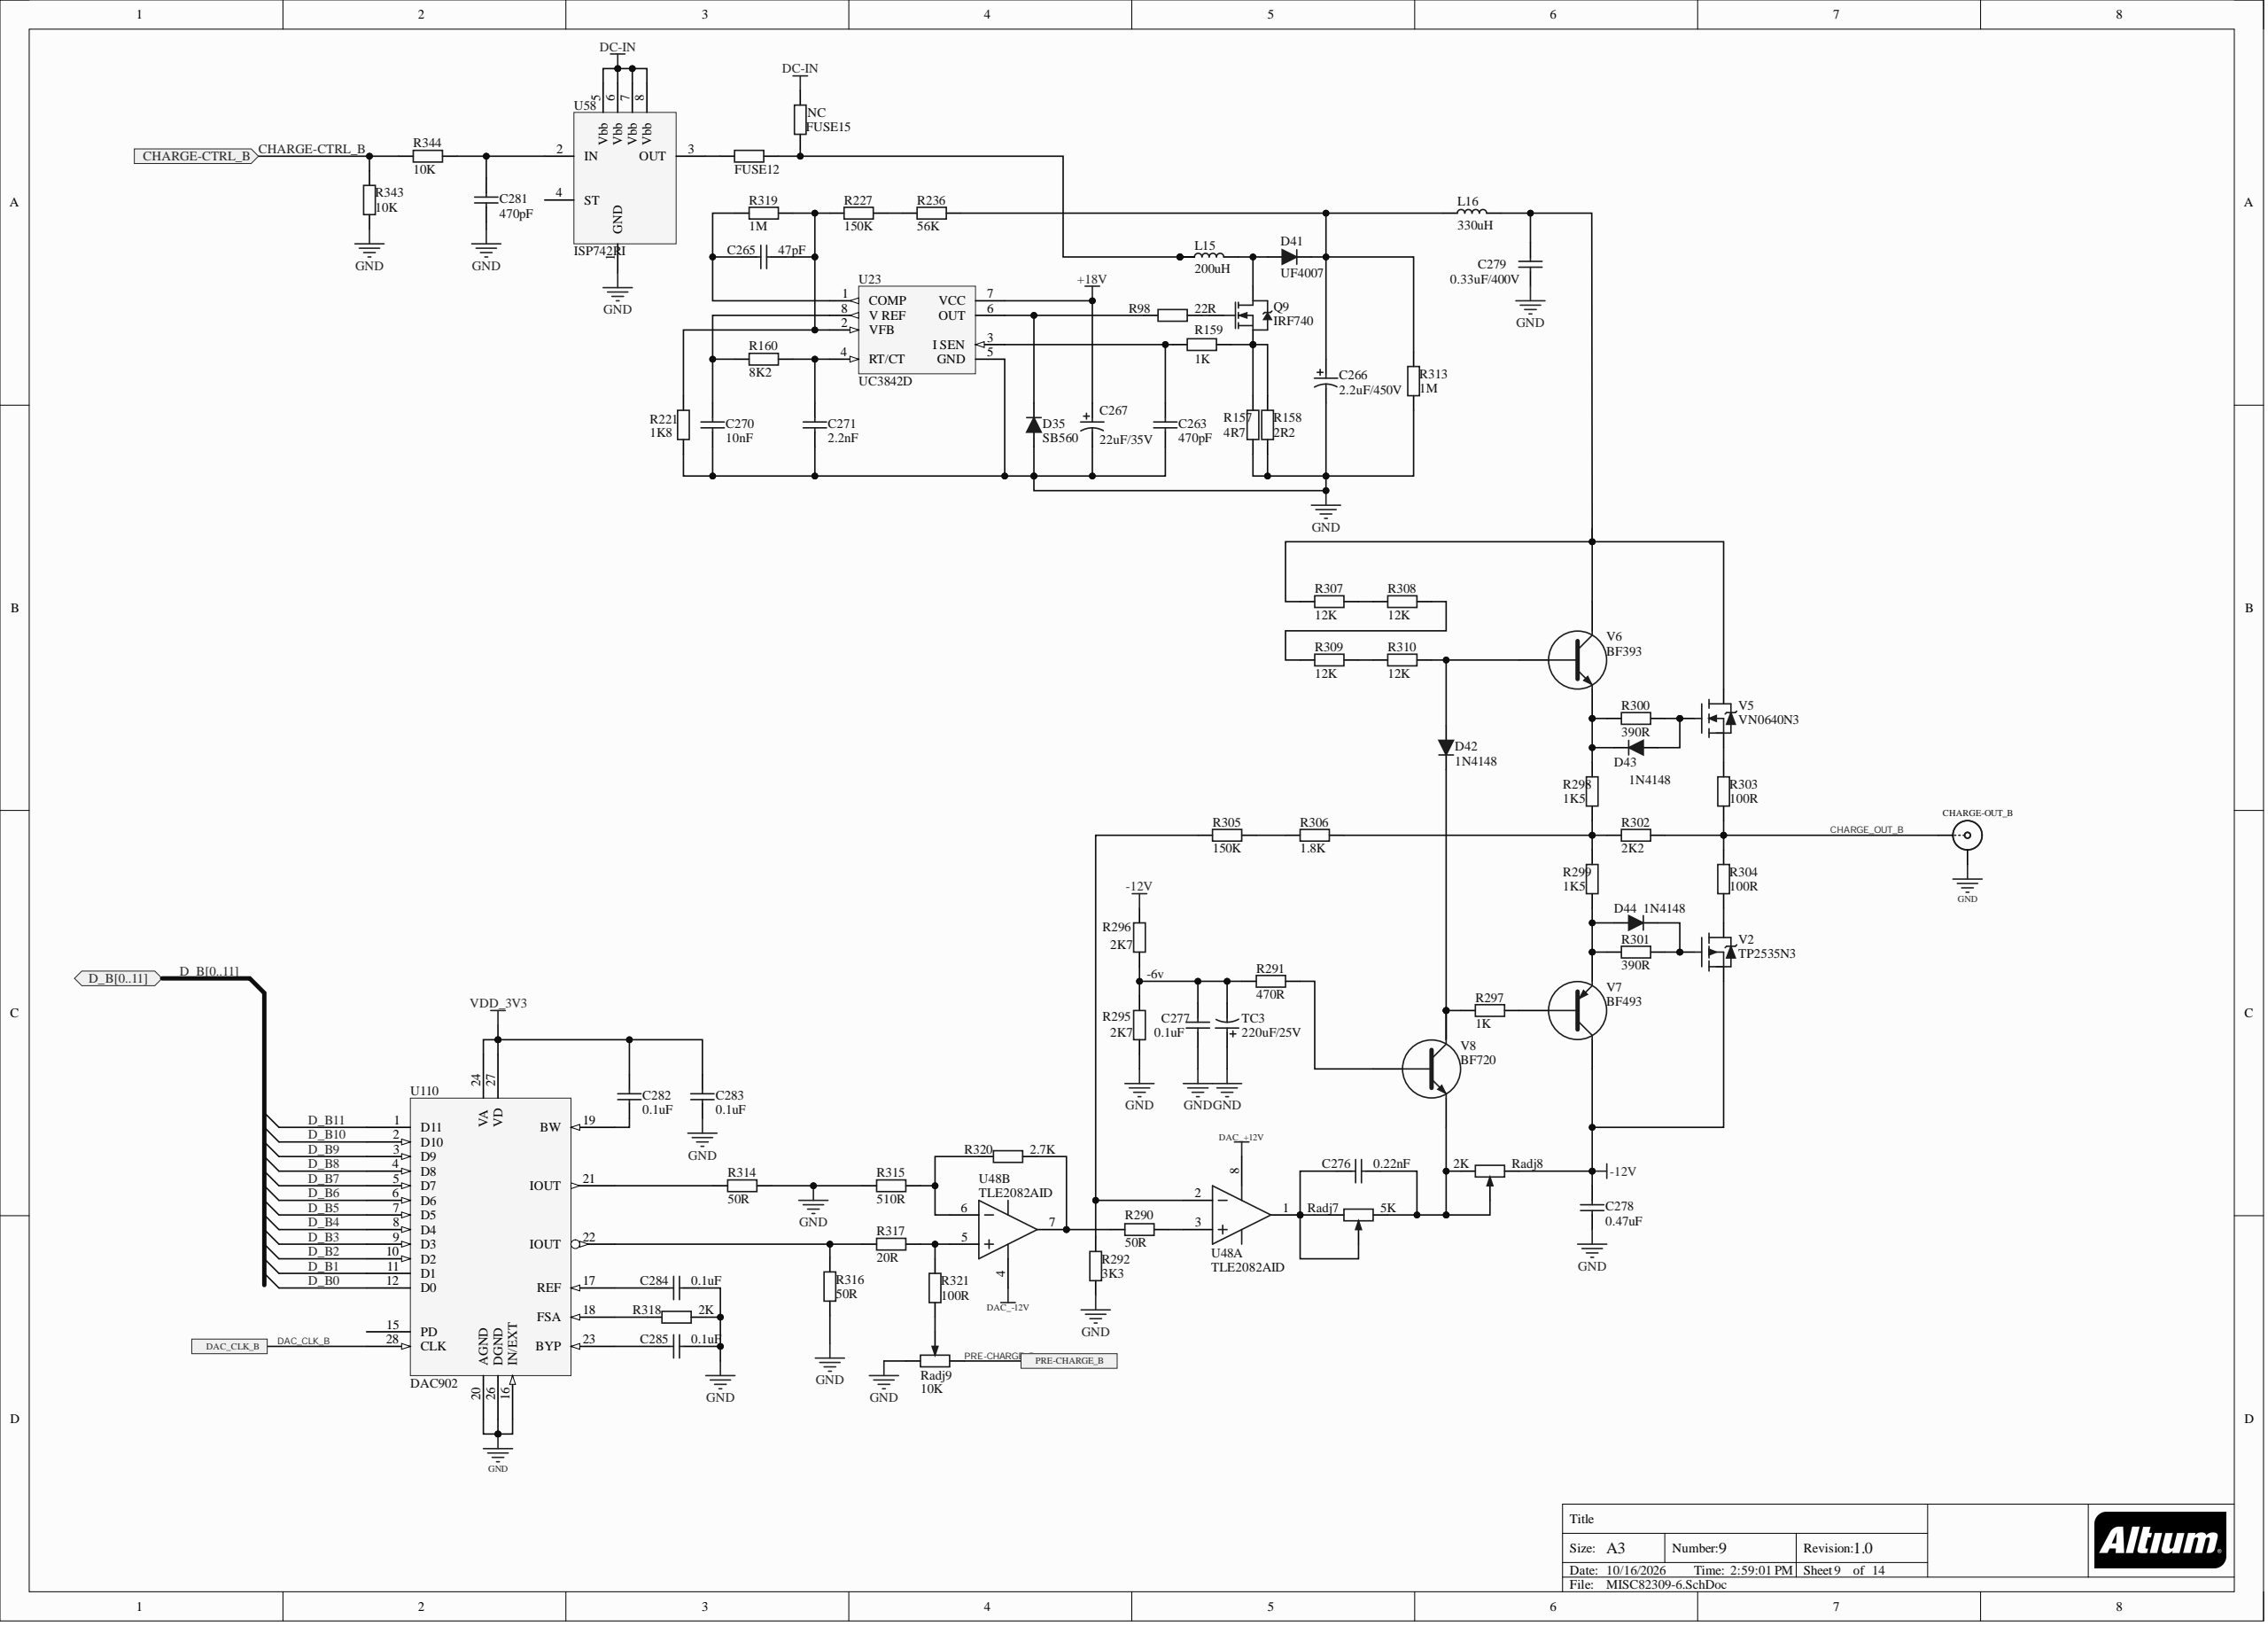Circuit board | Altium Designer | 747 parts | 576 nets | one sheet of the schematic
Parts on this sheet (reference | value | footprint):
C263 | 470pF | C1206
C265 | 47pF | C1206
C266 | 2.2uF/450V | CAP-EL-10X13_5-5
C267 | 22uF/35V | E6.3X5.4
C270 | 10nF | C1206
C271 | 2.2nF | C1206
C276 | 0.22nF | CAP_0805
C277 | 0.1uF | CAP_0805
C278 | 0.47uF | C1206
C279 | 0.33uF/400V | CBB-400V-10mm
C281 | 470pF | C0603
C282 | 0.1uF | CAP_0805
C283 | 0.1uF | CAP_0805
C284 | 0.1uF | CAP_0805
C285 | 0.1uF | CAP_0805
CHARGE-OUT_B | SMB | SMB_V-RJ45
D35 | SB560 | SB560
D41 | UF4007 | DO-41 - 10.46mm
D42 | 1N4148 | DO-213AA
D43 | 1N4148 | DO-213AA
D44 | 1N4148 | DO-213AA
FUSE12 | ASMD050-1812(30V,0.5A) | SMD1812-Fuse
FUSE15 | ASMD050-1812(30V,0.5A) | SMD1812-Fuse
L15 | 200uH | L200/1.4A
L16 | 330uH | L-9x12
Q9 | IRF740 | TO220V1
R98 | 22R | R1206
R157 | 4R7 | R1206
R158 | 2R2 | R1206
R159 | 1K | R1206
R160 | 8K2 | R1206
R221 | 1K8 | R1206
R227 | 150K | R1206
R236 | 56K | R1206
R290 | 50R | RES_0805
R291 | 470R | RES_0805
R292 | 3K3 | RES_0805
R295 | 2K7 | RES_0805
R296 | 2K7 | RES_0805
R297 | 1K | R1206
R298 | 1K5 | R1206
R299 | 1K5 | R1206
R300 | 390R | R1206
R301 | 390R | R1206
R302 | 2K2 | R1206
R303 | 100R | R1206
R304 | 100R | R1206
R305 | 150K | R1206
R306 | 1.8K | R1206
R307 | 12K | R1206
R308 | 12K | R1206
R309 | 12K | R1206
R310 | 12K | R1206
R313 | 1M | R1206
R314 | 50R | RES_0805
R315 | 510R | RES_0805
R316 | 50R | RES_0805
R317 | 20R | RES_0805
R318 | 2K | RES_0805
R319 | 1M | R1206
R320 | 2.7K | RES_0805
R321 | 100R | RES_0805
R343 | 10K | R0603
R344 | 10K | R0603
Radj7 | 5K | Radj
Radj8 | 2K | Radj
Radj9 | 10K | Radj
TC3 | 220uF/25V | E8X10,2
U23 | UC3842D | SOIC-8
U58 | ISP742RI | P-DSO-8
U110 | DAC902 | SOP127P1020X265-28N
V2 | TP2535N3 | TO-92
V5 | VN0640N3 | TO-92
V6 | BF393 | TO-92
V7 | BF493 | TO-92
V8 | BF720 | SOT223
Nets of these parts (net: part-pin ...):
VDD_3V3: C282-1 C283-1 U110-24 U110-27
PRE-CHARGE_B: Radj9-1
NetR321_1: R321-1 Radj9-2
NetR318_1: R318-1 U110-18
NetR317_2: R317-2 R321-2
NetR316_2: R316-2 R317-1 U110-22
NetR315_2: R315-2 R320-1
NetR314_1: R314-1 U110-21
NetR309_1: R309-1 R310-2
NetR308_1: R308-1 R309-2
NetR307_1: R307-1 R308-2
NetR305_1: R305-1 R306-2
NetR304_2: R304-2 V2-1
NetR303_1: R303-1 V5-1
NetR298_2: R298-2 R299-1 R302-1 R306-1
NetR297_1: R297-1 V7-2
NetR292_2: R292-2 R305-2
NetR291_1: R291-1 V8-1
NetR290_2: R290-2
NetR290_1: R290-1 R320-2
NetR227_2: R227-2 R236-1
NetQ9_3: Q9-3 R157-2 R158-2 R159-2
NetQ9_1: Q9-1 R98-2
NetFUSE12_2: FUSE12-2 FUSE15-2 L15-1 L15-3
NetFUSE12_1: FUSE12-1 U58-3
NetD44_2: D44-2 R301-2 V2-2
NetD44_1: D44-1 R299-2 R301-1 V7-1
NetD43_2: D43-2 R298-1 R300-1 V6-1
NetD43_1: D43-1 R300-2 V5-2
NetD42_2: D42-2 R297-2 V8-2 V8-4
NetD42_1: D42-1 R310-1 V6-2
NetD41_1: D41-1 L15-2 Q9-2
NetD35_2: D35-2 R98-1 U23-6
NetC285_2: C285-2 U110-23
NetC284_1: C284-1 U110-17
NetC282_2: C282-2 U110-19
NetC281_2: C281-2 R344-1 U58-2
NetC279_2: C279-2 L16-2 R307-2 V5-3 V6-3
NetC277_1: C277-1 R291-2 R295-1 R296-2 TC3-2
NetC276_2: C276-2 Radj7-1 Radj7-2
NetC276_1: C276-1 Radj7-3 Radj8-1 Radj8-2 V8-3
NetC271_1: C271-1 R160-2 U23-4
NetC270_1: C270-1 R160-1 U23-8
NetC266_1: C266-1 D41-2 L16-1 R236-2 R313-2
NetC265_2: C265-2 R319-1 U23-1
NetC265_1: C265-1 R221-2 R227-1 R319-2 U23-2
NetC263_1: C263-1 R159-1 U23-3
GND: C263-2 C266-2 C267-2 C270-2 C271-2 C277-2 C278-2 C279-1 C281-1 C283-2 C284-2 C285-1 CHARGE-OUT_B-2 D35-1 R157-1 R158-1 R221-1 R292-1 R295-2 R313-1 R314-2 R315-1 R316-1 R318-2 R343-1 Radj9-3 TC3-1 U23-5 U58-1 U110-16 U110-20 U110-26
DC-IN: FUSE15-1 U58-5 U58-6 U58-7 U58-8
DAC_CLK_B: U110-28
D_B11: U110-1
D_B10: U110-2
D_B9: U110-3
D_B8: U110-4
D_B7: U110-5
D_B6: U110-6
D_B5: U110-7
D_B4: U110-8
D_B3: U110-9
D_B2: U110-10
D_B1: U110-11
D_B0: U110-12
CHARGE_OUT_B: CHARGE-OUT_B-1 R302-2 R303-2 R304-1
CHARGE-CTRL_B: R343-2 R344-2
-12V: C278-1 R296-1 Radj8-3 V2-3 V7-3
+18V: C267-1 U23-7